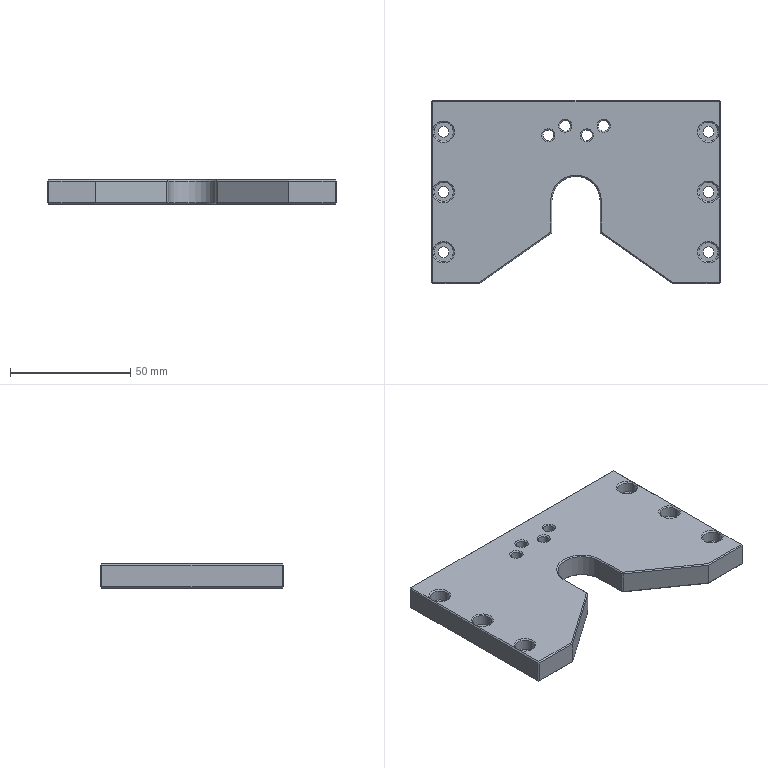Part | STEP file | Clip jig-top plate | 1 solid | 124 faces | box 120 x 76 x 10 mm | volume 73644 mm3 | plane 47 | cone 42 | cylinder 35 | commonest cylinder face diameters 4.5 x20 8 x12 2 x2 20 x1